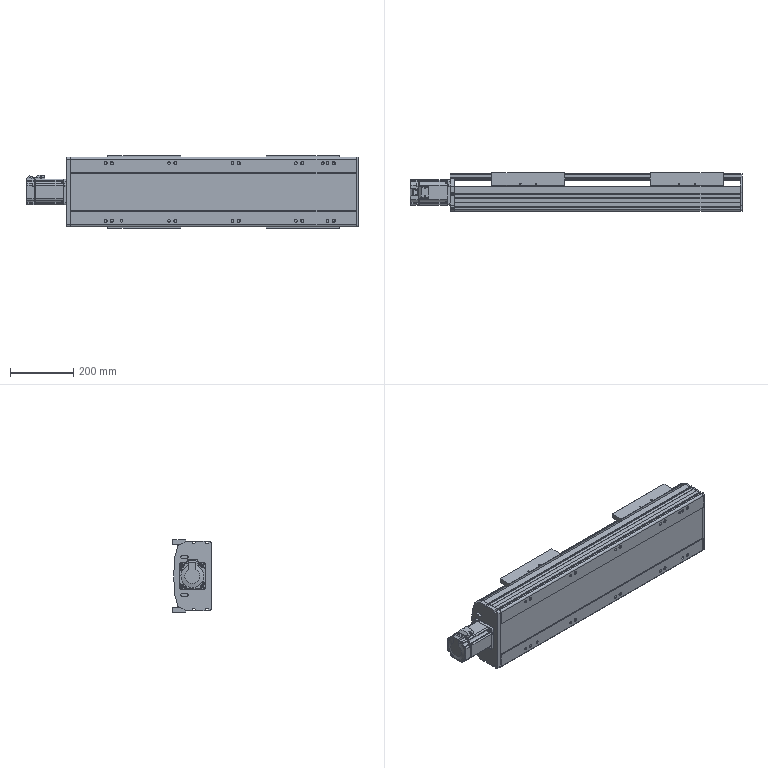Part | SolidWorks | features BaseBody 6, LPattern 1 | 7 solids | 1128 faces | box 1047 x 122 x 230 mm | volume 15190033 mm3 | plane 594 | cylinder 421 | cone 93 | spline 12 | torus 8 | commonest cylinder face diameters 8 x86 2 x32 6.647 x32 15 x28 0.6 x24 10 x22